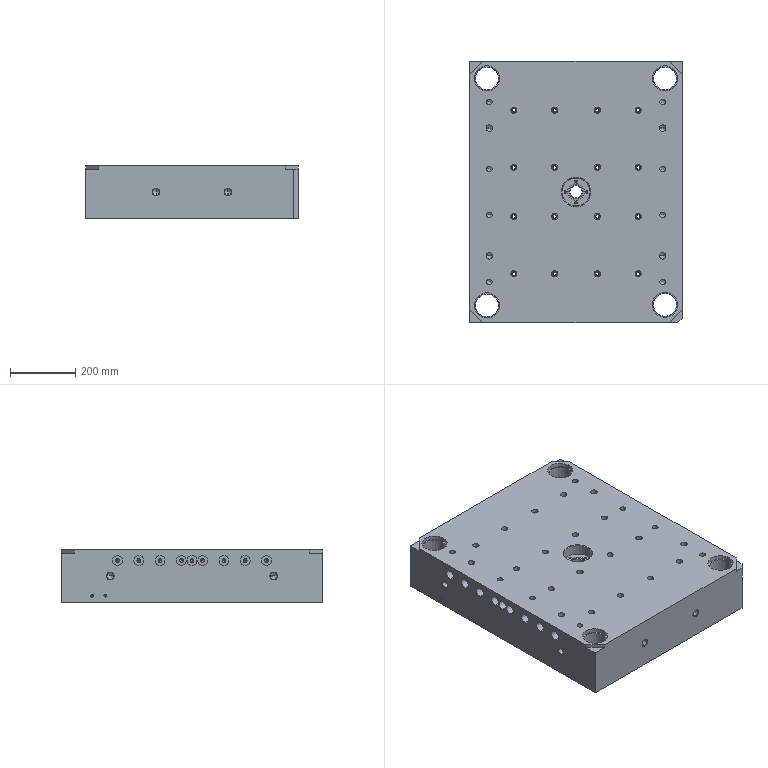Part | Creo | 1 solid | 1569 faces | box 650 x 800 x 160.003 mm | volume 48190432 mm3 | cylinder 783 | cone 536 | plane 242 | spline 8 | commonest cylinder face diameters 5.2 x160 6.8 x108 10 x104 6.799 x72 13 x68 21 x52